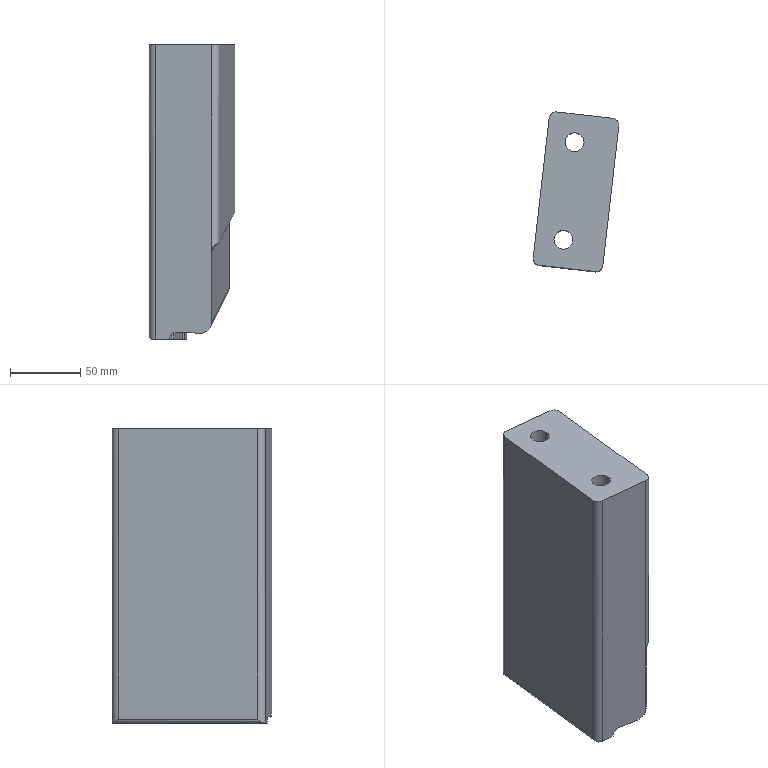Part | NX | features solid 2 | 1 solid | 30 faces | box 61.066 x 113.889 x 210 mm | volume 956028 mm3 | cylinder 15 | plane 14 | cone 1 | commonest cylinder face diameters 10 x7 13.5 x2 20 x2 6 x1 8.5 x1 9 x1
STEP:
#1=CARTESIAN_POINT('',(2372.499,-272.308,-109.613));
#2=VERTEX_POINT('',#1);
#3=CARTESIAN_POINT('',(2366.536,-324.649,-121.614));
#4=VERTEX_POINT('',#3);
#5=CARTESIAN_POINT('',(2363.422,-351.978,-127.881));
#6=DIRECTION('',(-0.1104,-0.9687,-0.2221));
#7=VECTOR('',#6,1000.);
#8=LINE('',#5,#7);
#9=EDGE_CURVE('',#2,#4,#8,.T.);
#10=ORIENTED_EDGE('',*,*,#9,.F.);
#11=CARTESIAN_POINT('',(2377.51,-274.226,-104.793));
#12=VERTEX_POINT('',#11);
#13=CARTESIAN_POINT('',(2372.499,-272.308,-109.613));
#14=CARTESIAN_POINT('',(2372.499,-272.308,-108.251));
#15=CARTESIAN_POINT('',(2373.556,-273.191,-105.664));
#16=CARTESIAN_POINT('',(2376.156,-274.098,-104.745));
#17=CARTESIAN_POINT('',(2377.51,-274.226,-104.793));
#18=B_SPLINE_CURVE_WITH_KNOTS('',3,(#13,#14,#15,#16,#17),.UNSPECIFIED.,.F.,.F.,(4,1,4),(0.,0.004026,0.008053),.UNSPECIFIED.);
#19=EDGE_CURVE('',#2,#12,#18,.T.);
#20=ORIENTED_EDGE('',*,*,#19,.T.);
#21=CARTESIAN_POINT('',(2371.85,-323.908,-116.185));
#22=VERTEX_POINT('',#21);
#23=CARTESIAN_POINT('',(2380.911,-244.376,-97.949));
#24=DIRECTION('',(0.1104,0.9687,0.2221));
#25=VECTOR('',#24,1000.);
#26=LINE('',#23,#25);
#27=EDGE_CURVE('',#22,#12,#26,.T.);
#28=ORIENTED_EDGE('',*,*,#27,.F.);
#29=CARTESIAN_POINT('',(2371.85,-323.908,-116.185));
#30=CARTESIAN_POINT('',(2370.434,-323.719,-116.122));
#31=CARTESIAN_POINT('',(2367.696,-324.057,-117.462));
#32=CARTESIAN_POINT('',(2366.536,-324.649,-120.186));
#33=CARTESIAN_POINT('',(2366.536,-324.649,-121.614));
#34=B_SPLINE_CURVE_WITH_KNOTS('',3,(#29,#30,#31,#32,#33),.UNSPECIFIED.,.F.,.F.,(4,1,4),(0.,0.004221,0.008443),.UNSPECIFIED.);
#35=EDGE_CURVE('',#22,#4,#34,.T.);
#36=ORIENTED_EDGE('',*,*,#35,.T.);
#37=EDGE_LOOP('',(#10,#20,#28,#36));
#38=FACE_BOUND('',#37,.T.);
#39=CARTESIAN_POINT('',(2377.356,-273.855,-109.838));
#40=DIRECTION('',(0.1104,0.9687,0.2221));
#41=DIRECTION('',(0.,0.2235,-0.9747));
#42=AXIS2_PLACEMENT_3D('',#39,#40,#41);
#43=CYLINDRICAL_SURFACE('',#42,5.);
#44=ADVANCED_FACE('',(#38),#43,.F.);
#45=CARTESIAN_POINT('',(2366.536,-324.649,-128.));
#46=VERTEX_POINT('',#45);
#47=CARTESIAN_POINT('',(2372.499,-272.308,-128.));
#48=VERTEX_POINT('',#47);
#49=CARTESIAN_POINT('',(2369.518,-298.479,-128.));
#50=DIRECTION('',(0.1132,0.9936,0.));
#51=VECTOR('',#50,1000.);
#52=LINE('',#49,#51);
#53=EDGE_CURVE('',#46,#48,#52,.T.);
#54=ORIENTED_EDGE('',*,*,#53,.T.);
#55=CARTESIAN_POINT('',(2372.499,-272.308,-101.));
#56=DIRECTION('',(0.,0.,1.));
#57=VECTOR('',#56,1000.);
#58=LINE('',#55,#57);
#59=EDGE_CURVE('',#48,#2,#58,.T.);
#60=ORIENTED_EDGE('',*,*,#59,.T.);
#61=ORIENTED_EDGE('',*,*,#9,.T.);
#62=CARTESIAN_POINT('',(2366.536,-324.649,-101.));
#63=DIRECTION('',(0.,0.,-1.));
#64=VECTOR('',#63,1000.);
#65=LINE('',#62,#64);
#66=EDGE_CURVE('',#4,#46,#65,.T.);
#67=ORIENTED_EDGE('',*,*,#66,.T.);
#68=EDGE_LOOP('',(#54,#60,#61,#67));
#69=FACE_BOUND('',#68,.T.);
#70=CARTESIAN_POINT('',(2369.518,-298.479,1.445));
#71=DIRECTION('',(-0.9936,0.1132,0.));
#72=DIRECTION('',(0.1132,0.9936,0.));
#73=AXIS2_PLACEMENT_3D('',#70,#71,#72);
#74=PLANE('',#73);
#75=ADVANCED_FACE('',(#69),#74,.F.);
#76=CARTESIAN_POINT('',(2363.363,-352.498,-128.));
#77=VERTEX_POINT('',#76);
#78=CARTESIAN_POINT('',(2364.575,-341.858,-128.));
#79=VERTEX_POINT('',#78);
#80=CARTESIAN_POINT('',(2369.518,-298.479,-128.));
#81=DIRECTION('',(0.1132,0.9936,0.));
#82=VECTOR('',#81,1000.);
#83=LINE('',#80,#82);
#84=EDGE_CURVE('',#77,#79,#83,.T.);
#85=ORIENTED_EDGE('',*,*,#84,.T.);
#86=CARTESIAN_POINT('',(2364.575,-341.858,-125.56));
#87=VERTEX_POINT('',#86);
#88=CARTESIAN_POINT('',(2364.575,-341.858,-101.));
#89=DIRECTION('',(0.,0.,1.));
#90=VECTOR('',#89,1000.);
#91=LINE('',#88,#90);
#92=EDGE_CURVE('',#79,#87,#91,.T.);
#93=ORIENTED_EDGE('',*,*,#92,.T.);
#94=CARTESIAN_POINT('',(2363.422,-351.978,-127.881));
#95=DIRECTION('',(-0.1104,-0.9687,-0.2221));
#96=VECTOR('',#95,1000.);
#97=LINE('',#94,#96);
#98=EDGE_CURVE('',#87,#77,#97,.T.);
#99=ORIENTED_EDGE('',*,*,#98,.T.);
#100=EDGE_LOOP('',(#85,#93,#99));
#101=FACE_BOUND('',#100,.T.);
#102=CARTESIAN_POINT('',(2369.518,-298.479,1.445));
#103=DIRECTION('',(-0.9936,0.1132,0.));
#104=DIRECTION('',(0.1132,0.9936,0.));
#105=AXIS2_PLACEMENT_3D('',#102,#103,#104);
#106=PLANE('',#105);
#107=ADVANCED_FACE('',(#101),#106,.F.);
#108=CARTESIAN_POINT('',(2379.774,-254.358,-100.238));
#109=VERTEX_POINT('',#108);
#110=CARTESIAN_POINT('',(2380.906,-244.421,-97.959));
#111=VERTEX_POINT('',#110);
#112=CARTESIAN_POINT('',(2380.911,-244.376,-97.949));
#113=DIRECTION('',(0.1104,0.9687,0.2221));
#114=VECTOR('',#113,1000.);
#115=LINE('',#112,#114);
#116=EDGE_CURVE('',#109,#111,#115,.T.);
#117=ORIENTED_EDGE('',*,*,#116,.F.);
#118=CARTESIAN_POINT('',(2374.46,-255.099,-105.667));
#119=VERTEX_POINT('',#118);
#120=CARTESIAN_POINT('',(2379.774,-254.358,-100.238));
#121=CARTESIAN_POINT('',(2378.358,-254.169,-100.174));
#122=CARTESIAN_POINT('',(2375.62,-254.507,-101.515));
#123=CARTESIAN_POINT('',(2374.46,-255.099,-104.238));
#124=CARTESIAN_POINT('',(2374.46,-255.099,-105.667));
#125=B_SPLINE_CURVE_WITH_KNOTS('',3,(#120,#121,#122,#123,#124),.UNSPECIFIED.,.F.,.F.,(4,1,4),(0.,0.004221,0.008443),.UNSPECIFIED.);
#126=EDGE_CURVE('',#109,#119,#125,.T.);
#127=ORIENTED_EDGE('',*,*,#126,.T.);
#128=CARTESIAN_POINT('',(2375.744,-243.832,-103.083));
#129=VERTEX_POINT('',#128);
#130=CARTESIAN_POINT('',(2363.422,-351.978,-127.881));
#131=DIRECTION('',(-0.1104,-0.9687,-0.2221));
#132=VECTOR('',#131,1000.);
#133=LINE('',#130,#132);
#134=EDGE_CURVE('',#129,#119,#133,.T.);
#135=ORIENTED_EDGE('',*,*,#134,.F.);
#136=CARTESIAN_POINT('',(2380.712,-244.398,-103.083));
#137=DIRECTION('',(-0.1132,-0.9936,0.));
#138=DIRECTION('',(0.,0.,1.));
#139=AXIS2_PLACEMENT_3D('',#136,#137,#138);
#140=ELLIPSE('',#139,5.128,5.);
#141=EDGE_CURVE('',#111,#129,#140,.T.);
#142=ORIENTED_EDGE('',*,*,#141,.F.);
#143=EDGE_LOOP('',(#117,#127,#135,#142));
#144=FACE_BOUND('',#143,.T.);
#145=CARTESIAN_POINT('',(2377.356,-273.855,-109.838));
#146=DIRECTION('',(0.1104,0.9687,0.2221));
#147=DIRECTION('',(0.,0.2235,-0.9747));
#148=AXIS2_PLACEMENT_3D('',#145,#146,#147);
#149=CYLINDRICAL_SURFACE('',#148,5.);
#150=ADVANCED_FACE('',(#144),#149,.F.);
#151=CARTESIAN_POINT('',(2393.099,-356.521,-118.358));
#152=VERTEX_POINT('',#151);
#153=CARTESIAN_POINT('',(2393.099,-356.521,82.));
#154=VERTEX_POINT('',#153);
#155=CARTESIAN_POINT('',(2393.099,-356.521,38.4));
#156=DIRECTION('',(0.,0.,1.));
#157=VECTOR('',#156,1000.);
#158=LINE('',#155,#157);
#159=EDGE_CURVE('',#152,#154,#158,.T.);
#160=ORIENTED_EDGE('',*,*,#159,.T.);
#161=CARTESIAN_POINT('',(2353.356,-351.993,82.));
#162=VERTEX_POINT('',#161);
#163=CARTESIAN_POINT('',(2417.456,-359.297,82.));
#164=DIRECTION('',(-0.9936,0.1132,0.));
#165=VECTOR('',#164,1000.);
#166=LINE('',#163,#165);
#167=EDGE_CURVE('',#154,#162,#166,.T.);
#168=ORIENTED_EDGE('',*,*,#167,.T.);
#169=CARTESIAN_POINT('',(2353.356,-351.993,-128.));
#170=VERTEX_POINT('',#169);
#171=CARTESIAN_POINT('',(2353.356,-351.993,-122.61));
#172=DIRECTION('',(0.,0.,-1.));
#173=VECTOR('',#172,1000.);
#174=LINE('',#171,#173);
#175=EDGE_CURVE('',#162,#170,#174,.T.);
#176=ORIENTED_EDGE('',*,*,#175,.T.);
#177=CARTESIAN_POINT('',(2363.293,-353.125,-128.));
#178=VERTEX_POINT('',#177);
#179=CARTESIAN_POINT('',(2417.456,-359.297,-128.));
#180=DIRECTION('',(-0.9936,0.1132,0.));
#181=VECTOR('',#180,1000.);
#182=LINE('',#179,#181);
#183=EDGE_CURVE('',#178,#170,#182,.T.);
#184=ORIENTED_EDGE('',*,*,#183,.F.);
#185=CARTESIAN_POINT('',(2368.454,-353.713,-123.02));
#186=VERTEX_POINT('',#185);
#187=CARTESIAN_POINT('',(2368.259,-353.691,-128.144));
#188=DIRECTION('',(0.1132,0.9936,0.));
#189=DIRECTION('',(0.,0.,1.));
#190=AXIS2_PLACEMENT_3D('',#187,#188,#189);
#191=ELLIPSE('',#190,5.128,5.);
#192=EDGE_CURVE('',#178,#186,#191,.T.);
#193=ORIENTED_EDGE('',*,*,#192,.T.);
#194=CARTESIAN_POINT('',(2385.336,-355.637,-123.702));
#195=VERTEX_POINT('',#194);
#196=CARTESIAN_POINT('',(2410.945,-358.555,-124.738));
#197=DIRECTION('',(-0.9928,0.1131,0.04014));
#198=VECTOR('',#197,1000.);
#199=LINE('',#196,#198);
#200=EDGE_CURVE('',#195,#186,#199,.T.);
#201=ORIENTED_EDGE('',*,*,#200,.F.);
#202=CARTESIAN_POINT('',(2385.647,-355.672,-115.504));
#203=DIRECTION('',(-0.1132,-0.9936,0.));
#204=DIRECTION('',(0.,0.,-1.));
#205=AXIS2_PLACEMENT_3D('',#202,#203,#204);
#206=ELLIPSE('',#205,8.205,8.);
#207=EDGE_CURVE('',#195,#152,#206,.T.);
#208=ORIENTED_EDGE('',*,*,#207,.T.);
#209=EDGE_LOOP('',(#160,#168,#176,#184,#193,#201,#208));
#210=FACE_BOUND('',#209,.T.);
#211=CARTESIAN_POINT('',(2417.456,-359.297,38.4));
#212=DIRECTION('',(0.1132,0.9936,0.));
#213=DIRECTION('',(0.,0.,1.));
#214=AXIS2_PLACEMENT_3D('',#211,#212,#213);
#215=PLANE('',#214);
#216=ADVANCED_FACE('',(#210),#215,.F.);
#217=CARTESIAN_POINT('',(2405.551,-247.228,82.));
#218=VERTEX_POINT('',#217);
#219=CARTESIAN_POINT('',(2365.808,-242.7,82.));
#220=VERTEX_POINT('',#219);
#221=CARTESIAN_POINT('',(2429.909,-250.004,82.));
#222=DIRECTION('',(-0.9936,0.1132,0.));
#223=VECTOR('',#222,1000.);
#224=LINE('',#221,#223);
#225=EDGE_CURVE('',#218,#220,#224,.T.);
#226=ORIENTED_EDGE('',*,*,#225,.F.);
#227=CARTESIAN_POINT('',(2405.551,-247.228,-93.298));
#228=VERTEX_POINT('',#227);
#229=CARTESIAN_POINT('',(2405.551,-247.228,-35.47));
#230=DIRECTION('',(0.,0.,-1.));
#231=VECTOR('',#230,1000.);
#232=LINE('',#229,#231);
#233=EDGE_CURVE('',#218,#228,#232,.T.);
#234=ORIENTED_EDGE('',*,*,#233,.T.);
#235=CARTESIAN_POINT('',(2397.788,-246.344,-98.642));
#236=VERTEX_POINT('',#235);
#237=CARTESIAN_POINT('',(2398.099,-246.379,-90.443));
#238=DIRECTION('',(-0.1132,-0.9936,0.));
#239=DIRECTION('',(0.,0.,-1.));
#240=AXIS2_PLACEMENT_3D('',#237,#238,#239);
#241=ELLIPSE('',#240,8.205,8.);
#242=EDGE_CURVE('',#236,#228,#241,.T.);
#243=ORIENTED_EDGE('',*,*,#242,.F.);
#244=CARTESIAN_POINT('',(2424.396,-249.376,-99.718));
#245=DIRECTION('',(-0.9928,0.1131,0.04014));
#246=VECTOR('',#245,1000.);
#247=LINE('',#244,#246);
#248=EDGE_CURVE('',#236,#111,#247,.T.);
#249=ORIENTED_EDGE('',*,*,#248,.T.);
#250=ORIENTED_EDGE('',*,*,#141,.T.);
#251=CARTESIAN_POINT('',(2375.744,-243.832,-128.));
#252=VERTEX_POINT('',#251);
#253=CARTESIAN_POINT('',(2375.744,-243.832,38.4));
#254=DIRECTION('',(0.,0.,1.));
#255=VECTOR('',#254,1000.);
#256=LINE('',#253,#255);
#257=EDGE_CURVE('',#252,#129,#256,.T.);
#258=ORIENTED_EDGE('',*,*,#257,.F.);
#259=CARTESIAN_POINT('',(2365.808,-242.7,-128.));
#260=VERTEX_POINT('',#259);
#261=CARTESIAN_POINT('',(2429.909,-250.004,-128.));
#262=DIRECTION('',(-0.9936,0.1132,0.));
#263=VECTOR('',#262,1000.);
#264=LINE('',#261,#263);
#265=EDGE_CURVE('',#252,#260,#264,.T.);
#266=ORIENTED_EDGE('',*,*,#265,.T.);
#267=CARTESIAN_POINT('',(2365.808,-242.7,38.4));
#268=DIRECTION('',(0.,0.,1.));
#269=VECTOR('',#268,1000.);
#270=LINE('',#267,#269);
#271=EDGE_CURVE('',#260,#220,#270,.T.);
#272=ORIENTED_EDGE('',*,*,#271,.T.);
#273=EDGE_LOOP('',(#226,#234,#243,#249,#250,#258,#266,#272));
#274=FACE_BOUND('',#273,.T.);
#275=CARTESIAN_POINT('',(2429.909,-250.004,38.4));
#276=DIRECTION('',(0.1132,0.9936,0.));
#277=DIRECTION('',(0.,0.,1.));
#278=AXIS2_PLACEMENT_3D('',#275,#276,#277);
#279=PLANE('',#278);
#280=ADVANCED_FACE('',(#274),#279,.T.);
#281=CARTESIAN_POINT('',(2409.953,-252.762,-36.609));
#282=VERTEX_POINT('',#281);
#283=CARTESIAN_POINT('',(2409.953,-252.762,82.));
#284=VERTEX_POINT('',#283);
#285=CARTESIAN_POINT('',(2409.953,-252.762,35.));
#286=DIRECTION('',(0.,0.,1.));
#287=VECTOR('',#286,1000.);
#288=LINE('',#285,#287);
#289=EDGE_CURVE('',#282,#284,#288,.T.);
#290=ORIENTED_EDGE('',*,*,#289,.T.);
#291=CARTESIAN_POINT('',(2398.633,-352.119,82.));
#292=VERTEX_POINT('',#291);
#293=CARTESIAN_POINT('',(2399.199,-347.152,82.));
#294=DIRECTION('',(-0.1132,-0.9936,0.));
#295=VECTOR('',#294,1000.);
#296=LINE('',#293,#295);
#297=EDGE_CURVE('',#284,#292,#296,.T.);
#298=ORIENTED_EDGE('',*,*,#297,.T.);
#299=CARTESIAN_POINT('',(2398.633,-352.119,-59.391));
#300=VERTEX_POINT('',#299);
#301=CARTESIAN_POINT('',(2398.633,-352.119,38.4));
#302=DIRECTION('',(0.,0.,-1.));
#303=VECTOR('',#302,1000.);
#304=LINE('',#301,#303);
#305=EDGE_CURVE('',#292,#300,#304,.T.);
#306=ORIENTED_EDGE('',*,*,#305,.T.);
#307=CARTESIAN_POINT('',(2401.568,-326.353,-53.483));
#308=DIRECTION('',(0.1104,0.9687,0.2221));
#309=VECTOR('',#308,1000.);
#310=LINE('',#307,#309);
#311=EDGE_CURVE('',#300,#282,#310,.T.);
#312=ORIENTED_EDGE('',*,*,#311,.T.);
#313=EDGE_LOOP('',(#290,#298,#306,#312));
#314=FACE_BOUND('',#313,.T.);
#315=CARTESIAN_POINT('',(2399.199,-347.152,38.4));
#316=DIRECTION('',(0.9936,-0.1132,0.));
#317=DIRECTION('',(-0.1132,-0.9936,0.));
#318=AXIS2_PLACEMENT_3D('',#315,#316,#317);
#319=PLANE('',#318);
#320=ADVANCED_FACE('',(#314),#319,.T.);
#321=ORIENTED_EDGE('',*,*,#233,.F.);
#322=CARTESIAN_POINT('',(2404.985,-252.196,82.));
#323=DIRECTION('',(0.,0.,-1.));
#324=DIRECTION('',(1.,0.,0.));
#325=AXIS2_PLACEMENT_3D('',#322,#323,#324);
#326=CIRCLE('',#325,5.);
#327=EDGE_CURVE('',#218,#284,#326,.T.);
#328=ORIENTED_EDGE('',*,*,#327,.T.);
#329=ORIENTED_EDGE('',*,*,#289,.F.);
#330=CARTESIAN_POINT('',(2409.957,-252.723,-36.6));
#331=VERTEX_POINT('',#330);
#332=CARTESIAN_POINT('',(2404.985,-252.196,-36.609));
#333=DIRECTION('',(0.02515,0.2207,-0.975));
#334=DIRECTION('',(-0.1104,-0.9687,-0.2221));
#335=AXIS2_PLACEMENT_3D('',#332,#333,#334);
#336=ELLIPSE('',#335,5.128,5.);
#337=EDGE_CURVE('',#331,#282,#336,.T.);
#338=ORIENTED_EDGE('',*,*,#337,.F.);
#339=CARTESIAN_POINT('',(2406.045,-247.31,-40.091));
#340=VERTEX_POINT('',#339);
#341=CARTESIAN_POINT('',(2406.045,-247.31,-40.091));
#342=CARTESIAN_POINT('',(2406.045,-247.31,-39.27));
#343=CARTESIAN_POINT('',(2406.446,-247.354,-37.641));
#344=CARTESIAN_POINT('',(2408.3,-248.195,-35.955));
#345=CARTESIAN_POINT('',(2409.846,-250.315,-36.028));
#346=CARTESIAN_POINT('',(2410.041,-251.926,-36.418));
#347=CARTESIAN_POINT('',(2409.957,-252.723,-36.6));
#348=B_SPLINE_CURVE_WITH_KNOTS('',3,(#341,#342,#343,#344,#345,#346,#347),.UNSPECIFIED.,.F.,.F.,(4,1,1,1,4),(0.,0.00243,0.004861,0.007291,0.009722),.UNSPECIFIED.);
#349=EDGE_CURVE('',#340,#331,#348,.T.);
#350=ORIENTED_EDGE('',*,*,#349,.F.);
#351=CARTESIAN_POINT('',(2406.045,-247.31,-90.449));
#352=VERTEX_POINT('',#351);
#353=CARTESIAN_POINT('',(2406.045,-247.31,-90.449));
#354=CARTESIAN_POINT('',(2406.045,-247.31,-87.116));
#355=CARTESIAN_POINT('',(2406.045,-247.31,-83.782));
#356=CARTESIAN_POINT('',(2406.045,-247.31,-66.996));
#357=CARTESIAN_POINT('',(2406.045,-247.31,-53.544));
#358=CARTESIAN_POINT('',(2406.045,-247.31,-40.091));
#359=B_SPLINE_CURVE_WITH_KNOTS('',3,(#353,#354,#355,#356,#357,#358),.UNSPECIFIED.,.F.,.F.,(4,2,4),(0.,0.1986,1.),.UNSPECIFIED.);
#360=EDGE_CURVE('',#352,#340,#359,.T.);
#361=ORIENTED_EDGE('',*,*,#360,.F.);
#362=CARTESIAN_POINT('',(2405.551,-247.228,-93.298));
#363=CARTESIAN_POINT('',(2405.881,-247.266,-92.38));
#364=CARTESIAN_POINT('',(2406.045,-247.31,-91.425));
#365=CARTESIAN_POINT('',(2406.045,-247.31,-90.449));
#366=B_SPLINE_CURVE_WITH_KNOTS('',3,(#362,#363,#364,#365),.UNSPECIFIED.,.F.,.F.,(4,4),(0.,0.002893),.UNSPECIFIED.);
#367=EDGE_CURVE('',#228,#352,#366,.T.);
#368=ORIENTED_EDGE('',*,*,#367,.F.);
#369=EDGE_LOOP('',(#321,#328,#329,#338,#350,#361,#368));
#370=FACE_BOUND('',#369,.T.);
#371=CARTESIAN_POINT('',(2404.985,-252.196,38.4));
#372=DIRECTION('',(0.,0.,-1.));
#373=DIRECTION('',(0.,-1.,0.));
#374=AXIS2_PLACEMENT_3D('',#371,#372,#373);
#375=CYLINDRICAL_SURFACE('',#374,5.);
#376=ADVANCED_FACE('',(#370),#375,.T.);
#377=ORIENTED_EDGE('',*,*,#305,.F.);
#378=CARTESIAN_POINT('',(2393.665,-351.553,82.));
#379=DIRECTION('',(0.,0.,-1.));
#380=DIRECTION('',(1.,0.,0.));
#381=AXIS2_PLACEMENT_3D('',#378,#379,#380);
#382=CIRCLE('',#381,5.);
#383=EDGE_CURVE('',#292,#154,#382,.T.);
#384=ORIENTED_EDGE('',*,*,#383,.T.);
#385=ORIENTED_EDGE('',*,*,#159,.F.);
#386=CARTESIAN_POINT('',(2393.598,-356.553,-115.498));
#387=VERTEX_POINT('',#386);
#388=CARTESIAN_POINT('',(2393.598,-356.553,-115.498));
#389=CARTESIAN_POINT('',(2393.598,-356.553,-116.477));
#390=CARTESIAN_POINT('',(2393.43,-356.559,-117.437));
#391=CARTESIAN_POINT('',(2393.099,-356.521,-118.358));
#392=B_SPLINE_CURVE_WITH_KNOTS('',3,(#388,#389,#390,#391),.UNSPECIFIED.,.F.,.F.,(4,4),(0.,0.002905),.UNSPECIFIED.);
#393=EDGE_CURVE('',#387,#152,#392,.T.);
#394=ORIENTED_EDGE('',*,*,#393,.F.);
#395=CARTESIAN_POINT('',(2393.598,-356.553,-65.14));
#396=VERTEX_POINT('',#395);
#397=CARTESIAN_POINT('',(2393.598,-356.553,-65.14));
#398=CARTESIAN_POINT('',(2393.598,-356.553,-68.473));
#399=CARTESIAN_POINT('',(2393.598,-356.553,-71.807));
#400=CARTESIAN_POINT('',(2393.598,-356.553,-88.593));
#401=CARTESIAN_POINT('',(2393.598,-356.553,-102.045));
#402=CARTESIAN_POINT('',(2393.598,-356.553,-115.498));
#403=B_SPLINE_CURVE_WITH_KNOTS('',3,(#397,#398,#399,#400,#401,#402),.UNSPECIFIED.,.F.,.F.,(4,2,4),(0.,0.1986,1.),.UNSPECIFIED.);
#404=EDGE_CURVE('',#396,#387,#403,.T.);
#405=ORIENTED_EDGE('',*,*,#404,.F.);
#406=CARTESIAN_POINT('',(2398.628,-352.159,-59.4));
#407=VERTEX_POINT('',#406);
#408=CARTESIAN_POINT('',(2398.628,-352.159,-59.4));
#409=CARTESIAN_POINT('',(2398.526,-352.99,-59.591));
#410=CARTESIAN_POINT('',(2397.908,-354.581,-59.936));
#411=CARTESIAN_POINT('',(2395.971,-356.186,-60.757));
#412=CARTESIAN_POINT('',(2394.07,-356.596,-62.585));
#413=CARTESIAN_POINT('',(2393.598,-356.553,-64.28));
#414=CARTESIAN_POINT('',(2393.598,-356.553,-65.14));
#415=B_SPLINE_CURVE_WITH_KNOTS('',3,(#408,#409,#410,#411,#412,#413,#414),.UNSPECIFIED.,.F.,.F.,(4,1,1,1,4),(0.,0.002539,0.005079,0.007618,0.01016),.UNSPECIFIED.);
#416=EDGE_CURVE('',#407,#396,#415,.T.);
#417=ORIENTED_EDGE('',*,*,#416,.F.);
#418=CARTESIAN_POINT('',(2393.665,-351.553,-59.391));
#419=DIRECTION('',(0.02515,0.2207,-0.975));
#420=DIRECTION('',(0.1104,0.9687,0.2221));
#421=AXIS2_PLACEMENT_3D('',#418,#419,#420);
#422=ELLIPSE('',#421,5.128,5.);
#423=EDGE_CURVE('',#300,#407,#422,.T.);
#424=ORIENTED_EDGE('',*,*,#423,.F.);
#425=EDGE_LOOP('',(#377,#384,#385,#394,#405,#417,#424));
#426=FACE_BOUND('',#425,.T.);
#427=CARTESIAN_POINT('',(2393.665,-351.553,38.4));
#428=DIRECTION('',(0.,0.,1.));
#429=DIRECTION('',(0.,1.,0.));
#430=AXIS2_PLACEMENT_3D('',#427,#428,#429);
#431=CYLINDRICAL_SURFACE('',#430,5.);
#432=ADVANCED_FACE('',(#426),#431,.T.);
#433=CARTESIAN_POINT('',(2360.274,-247.102,82.));
#434=VERTEX_POINT('',#433);
#435=CARTESIAN_POINT('',(2348.954,-346.459,82.));
#436=VERTEX_POINT('',#435);
#437=CARTESIAN_POINT('',(2349.52,-341.491,82.));
#438=DIRECTION('',(-0.1132,-0.9936,0.));
#439=VECTOR('',#438,1000.);
#440=LINE('',#437,#439);
#441=EDGE_CURVE('',#434,#436,#440,.T.);
#442=ORIENTED_EDGE('',*,*,#441,.F.);
#443=CARTESIAN_POINT('',(2360.274,-247.102,-125.));
#444=VERTEX_POINT('',#443);
#445=CARTESIAN_POINT('',(2360.274,-247.102,38.4));
#446=DIRECTION('',(0.,0.,-1.));
#447=VECTOR('',#446,1000.);
#448=LINE('',#445,#447);
#449=EDGE_CURVE('',#434,#444,#448,.T.);
#450=ORIENTED_EDGE('',*,*,#449,.T.);
#451=CARTESIAN_POINT('',(2348.954,-346.459,-125.));
#452=VERTEX_POINT('',#451);
#453=CARTESIAN_POINT('',(2349.52,-341.491,-125.));
#454=DIRECTION('',(-0.1132,-0.9936,0.));
#455=VECTOR('',#454,1000.);
#456=LINE('',#453,#455);
#457=EDGE_CURVE('',#444,#452,#456,.T.);
#458=ORIENTED_EDGE('',*,*,#457,.T.);
#459=CARTESIAN_POINT('',(2348.954,-346.459,35.));
#460=DIRECTION('',(0.,0.,1.));
#461=VECTOR('',#460,1000.);
#462=LINE('',#459,#461);
#463=EDGE_CURVE('',#452,#436,#462,.T.);
#464=ORIENTED_EDGE('',*,*,#463,.T.);
#465=EDGE_LOOP('',(#442,#450,#458,#464));
#466=FACE_BOUND('',#465,.T.);
#467=CARTESIAN_POINT('',(2349.52,-341.491,38.4));
#468=DIRECTION('',(0.9936,-0.1132,0.));
#469=DIRECTION('',(-0.1132,-0.9936,0.));
#470=AXIS2_PLACEMENT_3D('',#467,#468,#469);
#471=PLANE('',#470);
#472=ADVANCED_FACE('',(#466),#471,.F.);
#473=ORIENTED_EDGE('',*,*,#449,.F.);
#474=CARTESIAN_POINT('',(2365.242,-247.668,82.));
#475=DIRECTION('',(0.,0.,-1.));
#476=DIRECTION('',(1.,0.,0.));
#477=AXIS2_PLACEMENT_3D('',#474,#475,#476);
#478=CIRCLE('',#477,5.);
#479=EDGE_CURVE('',#434,#220,#478,.T.);
#480=ORIENTED_EDGE('',*,*,#479,.T.);
#481=ORIENTED_EDGE('',*,*,#271,.F.);
#482=CARTESIAN_POINT('',(2363.774,-242.889,-128.));
#483=VERTEX_POINT('',#482);
#484=CARTESIAN_POINT('',(2365.242,-247.668,-128.));
#485=DIRECTION('',(0.,0.,-1.));
#486=DIRECTION('',(-1.,0.,0.));
#487=AXIS2_PLACEMENT_3D('',#484,#485,#486);
#488=CIRCLE('',#487,5.);
#489=EDGE_CURVE('',#483,#260,#488,.T.);
#490=ORIENTED_EDGE('',*,*,#489,.F.);
#491=CARTESIAN_POINT('',(2363.774,-242.889,-128.));
#492=CARTESIAN_POINT('',(2362.701,-243.218,-128.));
#493=CARTESIAN_POINT('',(2360.996,-244.545,-127.03));
#494=CARTESIAN_POINT('',(2360.373,-246.235,-125.676));
#495=CARTESIAN_POINT('',(2360.274,-247.102,-125.));
#496=B_SPLINE_CURVE_WITH_KNOTS('',3,(#491,#492,#493,#494,#495),.UNSPECIFIED.,.F.,.F.,(4,1,4),(0.,0.00331,0.006621),.UNSPECIFIED.);
#497=EDGE_CURVE('',#483,#444,#496,.T.);
#498=ORIENTED_EDGE('',*,*,#497,.T.);
#499=EDGE_LOOP('',(#473,#480,#481,#490,#498));
#500=FACE_BOUND('',#499,.T.);
#501=CARTESIAN_POINT('',(2365.242,-247.668,38.4));
#502=DIRECTION('',(0.,0.,1.));
#503=DIRECTION('',(0.,1.,0.));
#504=AXIS2_PLACEMENT_3D('',#501,#502,#503);
#505=CYLINDRICAL_SURFACE('',#504,5.);
#506=ADVANCED_FACE('',(#500),#505,.T.);
#507=ORIENTED_EDGE('',*,*,#175,.F.);
#508=CARTESIAN_POINT('',(2353.922,-347.025,82.));
#509=DIRECTION('',(0.,0.,-1.));
#510=DIRECTION('',(1.,0.,0.));
#511=AXIS2_PLACEMENT_3D('',#508,#509,#510);
#512=CIRCLE('',#511,5.);
#513=EDGE_CURVE('',#162,#436,#512,.T.);
#514=ORIENTED_EDGE('',*,*,#513,.T.);
#515=ORIENTED_EDGE('',*,*,#463,.F.);
#516=CARTESIAN_POINT('',(2351.416,-351.352,-128.));
#517=VERTEX_POINT('',#516);
#518=CARTESIAN_POINT('',(2348.954,-346.459,-125.));
#519=CARTESIAN_POINT('',(2348.856,-347.321,-125.672));
#520=CARTESIAN_POINT('',(2349.076,-349.108,-127.028));
#521=CARTESIAN_POINT('',(2350.45,-350.793,-128.));
#522=CARTESIAN_POINT('',(2351.416,-351.352,-128.));
#523=B_SPLINE_CURVE_WITH_KNOTS('',3,(#518,#519,#520,#521,#522),.UNSPECIFIED.,.F.,.F.,(4,1,4),(-0.00001414,0.003277,0.006568),.UNSPECIFIED.);
#524=EDGE_CURVE('',#452,#517,#523,.T.);
#525=ORIENTED_EDGE('',*,*,#524,.T.);
#526=CARTESIAN_POINT('',(2353.922,-347.025,-128.));
#527=DIRECTION('',(0.,0.,-1.));
#528=DIRECTION('',(-1.,0.,0.));
#529=AXIS2_PLACEMENT_3D('',#526,#527,#528);
#530=CIRCLE('',#529,5.);
#531=EDGE_CURVE('',#170,#517,#530,.T.);
#532=ORIENTED_EDGE('',*,*,#531,.F.);
#533=EDGE_LOOP('',(#507,#514,#515,#525,#532));
#534=FACE_BOUND('',#533,.T.);
#535=CARTESIAN_POINT('',(2353.922,-347.025,38.4));
#536=DIRECTION('',(0.,0.,-1.));
#537=DIRECTION('',(0.,-1.,0.));
#538=AXIS2_PLACEMENT_3D('',#535,#536,#537);
#539=CYLINDRICAL_SURFACE('',#538,5.);
#540=ADVANCED_FACE('',(#534),#539,.T.);
#541=CARTESIAN_POINT('',(2380.805,-294.592,-109.543));
#542=VERTEX_POINT('',#541);
#543=CARTESIAN_POINT('',(2381.064,-298.834,-110.526));
#544=DIRECTION('',(0.01376,-0.225,0.9743));
#545=DIRECTION('',(-0.05948,0.9725,0.2254));
#546=AXIS2_PLACEMENT_3D('',#543,#544,#545);
#547=ELLIPSE('',#546,4.362,4.25);
#548=EDGE_CURVE('',#542,#542,#547,.T.);
#549=ORIENTED_EDGE('',*,*,#548,.T.);
#550=EDGE_LOOP('',(#549));
#551=FACE_BOUND('',#550,.T.);
#552=ORIENTED_EDGE('',*,*,#27,.T.);
#553=CARTESIAN_POINT('',(2378.448,-264.27,-102.508));
#554=DIRECTION('',(0.01376,-0.225,0.9743));
#555=DIRECTION('',(-0.05948,0.9725,0.2254));
#556=AXIS2_PLACEMENT_3D('',#553,#554,#555);
#557=ELLIPSE('',#556,10.264,10.);
#558=EDGE_CURVE('',#12,#109,#557,.T.);
#559=ORIENTED_EDGE('',*,*,#558,.T.);
#560=ORIENTED_EDGE('',*,*,#116,.T.);
#561=ORIENTED_EDGE('',*,*,#248,.F.);
#562=CARTESIAN_POINT('',(2399.334,-232.771,-95.53));
#563=DIRECTION('',(-0.1104,-0.9687,-0.2221));
#564=VECTOR('',#563,1000.);
#565=LINE('',#562,#564);
#566=EDGE_CURVE('',#236,#195,#565,.T.);
#567=ORIENTED_EDGE('',*,*,#566,.T.);
#568=ORIENTED_EDGE('',*,*,#200,.T.);
#569=CARTESIAN_POINT('',(2369.586,-343.776,-120.741));
#570=VERTEX_POINT('',#569);
#571=CARTESIAN_POINT('',(2380.911,-244.376,-97.949));
#572=DIRECTION('',(0.1104,0.9687,0.2221));
#573=VECTOR('',#572,1000.);
#574=LINE('',#571,#573);
#575=EDGE_CURVE('',#186,#570,#574,.T.);
#576=ORIENTED_EDGE('',*,*,#575,.T.);
#577=CARTESIAN_POINT('',(2370.523,-333.82,-118.455));
#578=DIRECTION('',(0.01376,-0.225,0.9743));
#579=DIRECTION('',(-0.05948,0.9725,0.2254));
#580=AXIS2_PLACEMENT_3D('',#577,#578,#579);
#581=ELLIPSE('',#580,10.264,10.);
#582=EDGE_CURVE('',#570,#22,#581,.T.);
#583=ORIENTED_EDGE('',*,*,#582,.T.);
#584=EDGE_LOOP('',(#552,#559,#560,#561,#567,#568,#576,#583));
#585=FACE_BOUND('',#584,.T.);
#586=CARTESIAN_POINT('',(2436.542,-222.854,-93.765));
#587=DIRECTION('',(0.01376,-0.225,0.9743));
#588=DIRECTION('',(-0.05948,0.9725,0.2254));
#589=AXIS2_PLACEMENT_3D('',#586,#587,#588);
#590=PLANE('',#589);
#591=ADVANCED_FACE('',(#551,#585),#590,.F.);
#592=CARTESIAN_POINT('',(2393.099,-360.929,-116.501));
#593=DIRECTION('',(0.1104,0.9687,0.2221));
#594=VECTOR('',#593,1000.);
#595=LINE('',#592,#594);
#596=EDGE_CURVE('',#387,#352,#595,.T.);
#597=ORIENTED_EDGE('',*,*,#596,.F.);
#598=ORIENTED_EDGE('',*,*,#393,.T.);
#599=ORIENTED_EDGE('',*,*,#207,.F.);
#600=ORIENTED_EDGE('',*,*,#566,.F.);
#601=ORIENTED_EDGE('',*,*,#242,.T.);
#602=ORIENTED_EDGE('',*,*,#367,.T.);
#603=EDGE_LOOP('',(#597,#598,#599,#600,#601,#602));
#604=FACE_BOUND('',#603,.T.);
#605=CARTESIAN_POINT('',(2401.001,-220.905,-84.602));
#606=DIRECTION('',(-0.1104,-0.9687,-0.2221));
#607=DIRECTION('',(0.,0.2235,-0.9747));
#608=AXIS2_PLACEMENT_3D('',#605,#606,#607);
#609=CYLINDRICAL_SURFACE('',#608,8.);
#610=ADVANCED_FACE('',(#604),#609,.T.);
#611=CARTESIAN_POINT('',(2407.715,-232.647,-36.729));
#612=DIRECTION('',(-0.1104,-0.9687,-0.2221));
#613=VECTOR('',#612,1000.);
#614=LINE('',#611,#613);
#615=EDGE_CURVE('',#340,#396,#614,.T.);
#616=ORIENTED_EDGE('',*,*,#615,.T.);
#617=ORIENTED_EDGE('',*,*,#404,.T.);
#618=ORIENTED_EDGE('',*,*,#596,.T.);
#619=ORIENTED_EDGE('',*,*,#360,.T.);
#620=EDGE_LOOP('',(#616,#617,#618,#619));
#621=FACE_BOUND('',#620,.T.);
#622=CARTESIAN_POINT('',(2407.602,-233.641,-32.341));
#623=DIRECTION('',(-0.9936,0.1132,0.000000002));
#624=DIRECTION('',(0.1132,0.9936,0.000000002));
#625=AXIS2_PLACEMENT_3D('',#622,#623,#624);
#626=PLANE('',#625);
#627=ADVANCED_FACE('',(#621),#626,.F.);
#628=CARTESIAN_POINT('',(2397.78,-359.603,-61.107));
#629=DIRECTION('',(0.1104,0.9687,0.2221));
#630=VECTOR('',#629,1000.);
#631=LINE('',#628,#630);
#632=EDGE_CURVE('',#407,#331,#631,.T.);
#633=ORIENTED_EDGE('',*,*,#632,.F.);
#634=ORIENTED_EDGE('',*,*,#416,.T.);
#635=ORIENTED_EDGE('',*,*,#615,.F.);
#636=ORIENTED_EDGE('',*,*,#349,.T.);
#637=EDGE_LOOP('',(#633,#634,#635,#636));
#638=FACE_BOUND('',#637,.T.);
#639=CARTESIAN_POINT('',(2397.059,-365.932,-67.174));
#640=DIRECTION('',(0.1104,0.9687,0.2221));
#641=DIRECTION('',(0.,-0.2235,0.9747));
#642=AXIS2_PLACEMENT_3D('',#639,#640,#641);
#643=CYLINDRICAL_SURFACE('',#642,4.5);
#644=ADVANCED_FACE('',(#638),#643,.F.);
#645=ORIENTED_EDGE('',*,*,#311,.F.);
#646=ORIENTED_EDGE('',*,*,#423,.T.);
#647=ORIENTED_EDGE('',*,*,#632,.T.);
#648=ORIENTED_EDGE('',*,*,#337,.T.);
#649=EDGE_LOOP('',(#645,#646,#647,#648));
#650=FACE_BOUND('',#649,.T.);
#651=CARTESIAN_POINT('',(2449.123,-372.87,-62.786));
#652=DIRECTION('',(0.02515,0.2207,-0.975));
#653=DIRECTION('',(-0.1104,-0.9687,-0.2221));
#654=AXIS2_PLACEMENT_3D('',#651,#652,#653);
#655=PLANE('',#654);
#656=ADVANCED_FACE('',(#650),#655,.T.);
#657=ORIENTED_EDGE('',*,*,#134,.T.);
#658=CARTESIAN_POINT('',(2374.46,-255.099,-128.));
#659=VERTEX_POINT('',#658);
#660=CARTESIAN_POINT('',(2374.46,-255.099,-101.));
#661=DIRECTION('',(0.,0.,-1.));
#662=VECTOR('',#661,1000.);
#663=LINE('',#660,#662);
#664=EDGE_CURVE('',#119,#659,#663,.T.);
#665=ORIENTED_EDGE('',*,*,#664,.T.);
#666=CARTESIAN_POINT('',(2369.518,-298.479,-128.));
#667=DIRECTION('',(0.1132,0.9936,0.));
#668=VECTOR('',#667,1000.);
#669=LINE('',#666,#668);
#670=EDGE_CURVE('',#659,#252,#669,.T.);
#671=ORIENTED_EDGE('',*,*,#670,.T.);
#672=ORIENTED_EDGE('',*,*,#257,.T.);
#673=EDGE_LOOP('',(#657,#665,#671,#672));
#674=FACE_BOUND('',#673,.T.);
#675=CARTESIAN_POINT('',(2369.518,-298.479,1.445));
#676=DIRECTION('',(-0.9936,0.1132,0.));
#677=DIRECTION('',(0.1132,0.9936,0.));
#678=AXIS2_PLACEMENT_3D('',#675,#676,#677);
#679=PLANE('',#678);
#680=ADVANCED_FACE('',(#674),#679,.F.);
#681=ORIENTED_EDGE('',*,*,#497,.F.);
#682=CARTESIAN_POINT('',(2369.029,-196.759,-128.));
#683=DIRECTION('',(0.1132,0.9936,0.));
#684=VECTOR('',#683,1000.);
#685=LINE('',#682,#684);
#686=EDGE_CURVE('',#517,#483,#685,.T.);
#687=ORIENTED_EDGE('',*,*,#686,.F.);
#688=ORIENTED_EDGE('',*,*,#524,.F.);
#689=ORIENTED_EDGE('',*,*,#457,.F.);
#690=EDGE_LOOP('',(#681,#687,#688,#689));
#691=FACE_BOUND('',#690,.T.);
#692=CARTESIAN_POINT('',(2369.029,-196.759,-125.));
#693=DIRECTION('',(-0.1132,-0.9936,0.));
#694=DIRECTION('',(-0.9936,0.1132,0.));
#695=AXIS2_PLACEMENT_3D('',#692,#693,#694);
#696=CYLINDRICAL_SURFACE('',#695,3.);
#697=ADVANCED_FACE('',(#691),#696,.T.);
#698=ORIENTED_EDGE('',*,*,#670,.F.);
#699=CARTESIAN_POINT('',(2378.448,-264.27,-128.));
#700=DIRECTION('',(0.,0.,1.));
#701=DIRECTION('',(-1.,0.,0.));
#702=AXIS2_PLACEMENT_3D('',#699,#700,#701);
#703=CIRCLE('',#702,10.);
#704=EDGE_CURVE('',#659,#48,#703,.T.);
#705=ORIENTED_EDGE('',*,*,#704,.T.);
#706=ORIENTED_EDGE('',*,*,#53,.F.);
#707=CARTESIAN_POINT('',(2370.523,-333.82,-128.));
#708=DIRECTION('',(0.,0.,1.));
#709=DIRECTION('',(-1.,0.,0.));
#710=AXIS2_PLACEMENT_3D('',#707,#708,#709);
#711=CIRCLE('',#710,10.);
#712=EDGE_CURVE('',#46,#79,#711,.T.);
#713=ORIENTED_EDGE('',*,*,#712,.T.);
#714=ORIENTED_EDGE('',*,*,#84,.F.);
#715=CARTESIAN_POINT('',(2368.331,-353.064,-128.));
#716=DIRECTION('',(0.,0.,1.));
#717=DIRECTION('',(0.1132,0.9936,0.));
#718=AXIS2_PLACEMENT_3D('',#715,#716,#717);
#719=ELLIPSE('',#718,22.509,5.);
#720=EDGE_CURVE('',#77,#178,#719,.T.);
#721=ORIENTED_EDGE('',*,*,#720,.T.);
#722=ORIENTED_EDGE('',*,*,#183,.T.);
#723=ORIENTED_EDGE('',*,*,#531,.T.);
#724=ORIENTED_EDGE('',*,*,#686,.T.);
#725=ORIENTED_EDGE('',*,*,#489,.T.);
#726=ORIENTED_EDGE('',*,*,#265,.F.);
#727=EDGE_LOOP('',(#698,#705,#706,#713,#714,#721,#722,#723,#724,#725,#726));
#728=FACE_BOUND('',#727,.T.);
#729=CARTESIAN_POINT('',(2535.468,-215.723,-128.));
#730=DIRECTION('',(0.,0.,-1.));
#731=DIRECTION('',(-0.1132,-0.9936,0.));
#732=AXIS2_PLACEMENT_3D('',#729,#730,#731);
#733=PLANE('',#732);
#734=ADVANCED_FACE('',(#728),#733,.T.);
#735=ORIENTED_EDGE('',*,*,#98,.F.);
#736=CARTESIAN_POINT('',(2364.575,-341.858,-125.56));
#737=CARTESIAN_POINT('',(2364.575,-341.858,-124.199));
#738=CARTESIAN_POINT('',(2365.632,-342.741,-121.611));
#739=CARTESIAN_POINT('',(2368.232,-343.648,-120.692));
#740=CARTESIAN_POINT('',(2369.586,-343.776,-120.741));
#741=B_SPLINE_CURVE_WITH_KNOTS('',3,(#736,#737,#738,#739,#740),.UNSPECIFIED.,.F.,.F.,(4,1,4),(0.,0.004026,0.008053),.UNSPECIFIED.);
#742=EDGE_CURVE('',#87,#570,#741,.T.);
#743=ORIENTED_EDGE('',*,*,#742,.T.);
#744=ORIENTED_EDGE('',*,*,#575,.F.);
#745=ORIENTED_EDGE('',*,*,#192,.F.);
#746=ORIENTED_EDGE('',*,*,#720,.F.);
#747=EDGE_LOOP('',(#735,#743,#744,#745,#746));
#748=FACE_BOUND('',#747,.T.);
#749=CARTESIAN_POINT('',(2377.356,-273.855,-109.838));
#750=DIRECTION('',(0.1104,0.9687,0.2221));
#751=DIRECTION('',(0.,0.2235,-0.9747));
#752=AXIS2_PLACEMENT_3D('',#749,#750,#751);
#753=CYLINDRICAL_SURFACE('',#752,5.);
#754=ADVANCED_FACE('',(#748),#753,.F.);
#755=CARTESIAN_POINT('',(2385.198,-264.27,82.));
#756=VERTEX_POINT('',#755);
#757=CARTESIAN_POINT('',(2378.448,-264.27,82.));
#758=DIRECTION('',(0.,0.,1.));
#759=DIRECTION('',(1.,0.,0.));
#760=AXIS2_PLACEMENT_3D('',#757,#758,#759);
#761=CIRCLE('',#760,6.75);
#762=EDGE_CURVE('',#756,#756,#761,.T.);
#763=ORIENTED_EDGE('',*,*,#762,.F.);
#764=EDGE_LOOP('',(#763));
#765=FACE_BOUND('',#764,.T.);
#766=CARTESIAN_POINT('',(2377.273,-333.82,82.));
#767=VERTEX_POINT('',#766);
#768=CARTESIAN_POINT('',(2370.523,-333.82,82.));
#769=DIRECTION('',(0.,0.,1.));
#770=DIRECTION('',(1.,0.,0.));
#771=AXIS2_PLACEMENT_3D('',#768,#769,#770);
#772=CIRCLE('',#771,6.75);
#773=EDGE_CURVE('',#767,#767,#772,.T.);
#774=ORIENTED_EDGE('',*,*,#773,.F.);
#775=EDGE_LOOP('',(#774));
#776=FACE_BOUND('',#775,.T.);
#777=ORIENTED_EDGE('',*,*,#327,.F.);
#778=ORIENTED_EDGE('',*,*,#225,.T.);
#779=ORIENTED_EDGE('',*,*,#479,.F.);
#780=ORIENTED_EDGE('',*,*,#441,.T.);
#781=ORIENTED_EDGE('',*,*,#513,.F.);
#782=ORIENTED_EDGE('',*,*,#167,.F.);
#783=ORIENTED_EDGE('',*,*,#383,.F.);
#784=ORIENTED_EDGE('',*,*,#297,.F.);
#785=EDGE_LOOP('',(#777,#778,#779,#780,#781,#782,#783,#784));
#786=FACE_BOUND('',#785,.T.);
#787=CARTESIAN_POINT('',(2439.558,-260.55,82.));
#788=DIRECTION('',(0.,0.,1.));
#789=DIRECTION('',(-1.,0.,0.));
#790=AXIS2_PLACEMENT_3D('',#787,#788,#789);
#791=PLANE('',#790);
#792=ADVANCED_FACE('',(#765,#776,#786),#791,.T.);
#793=CARTESIAN_POINT('',(2380.523,-333.82,2.));
#794=VERTEX_POINT('',#793);
#795=CARTESIAN_POINT('',(2370.523,-333.82,2.));
#796=DIRECTION('',(0.,0.,-1.));
#797=DIRECTION('',(1.,0.,0.));
#798=AXIS2_PLACEMENT_3D('',#795,#796,#797);
#799=CIRCLE('',#798,10.);
#800=EDGE_CURVE('',#794,#794,#799,.T.);
#801=ORIENTED_EDGE('',*,*,#800,.F.);
#802=EDGE_LOOP('',(#801));
#803=FACE_BOUND('',#802,.T.);
#804=ORIENTED_EDGE('',*,*,#35,.F.);
#805=ORIENTED_EDGE('',*,*,#582,.F.);
#806=ORIENTED_EDGE('',*,*,#742,.F.);
#807=ORIENTED_EDGE('',*,*,#92,.F.);
#808=ORIENTED_EDGE('',*,*,#712,.F.);
#809=ORIENTED_EDGE('',*,*,#66,.F.);
#810=EDGE_LOOP('',(#804,#805,#806,#807,#808,#809));
#811=FACE_BOUND('',#810,.T.);
#812=CARTESIAN_POINT('',(2370.523,-333.82,-101.));
#813=DIRECTION('',(0.,0.,1.));
#814=DIRECTION('',(-0.9744,0.225,0.));
#815=AXIS2_PLACEMENT_3D('',#812,#813,#814);
#816=CYLINDRICAL_SURFACE('',#815,10.);
#817=ADVANCED_FACE('',(#803,#811),#816,.F.);
#818=ORIENTED_EDGE('',*,*,#773,.T.);
#819=EDGE_LOOP('',(#818));
#820=FACE_BOUND('',#819,.T.);
#821=CARTESIAN_POINT('',(2377.273,-333.82,2.));
#822=VERTEX_POINT('',#821);
#823=CARTESIAN_POINT('',(2370.523,-333.82,2.));
#824=DIRECTION('',(0.,0.,-1.));
#825=DIRECTION('',(1.,0.,0.));
#826=AXIS2_PLACEMENT_3D('',#823,#824,#825);
#827=CIRCLE('',#826,6.75);
#828=EDGE_CURVE('',#822,#822,#827,.T.);
#829=ORIENTED_EDGE('',*,*,#828,.T.);
#830=EDGE_LOOP('',(#829));
#831=FACE_BOUND('',#830,.T.);
#832=CARTESIAN_POINT('',(2370.523,-333.82,-101.));
#833=DIRECTION('',(0.,0.,1.));
#834=DIRECTION('',(-0.9744,0.225,0.));
#835=AXIS2_PLACEMENT_3D('',#832,#833,#834);
#836=CYLINDRICAL_SURFACE('',#835,6.75);
#837=ADVANCED_FACE('',(#820,#831),#836,.F.);
#838=ORIENTED_EDGE('',*,*,#828,.F.);
#839=EDGE_LOOP('',(#838));
#840=FACE_BOUND('',#839,.T.);
#841=ORIENTED_EDGE('',*,*,#800,.T.);
#842=EDGE_LOOP('',(#841));
#843=FACE_BOUND('',#842,.T.);
#844=CARTESIAN_POINT('',(2439.558,-260.55,2.));
#845=DIRECTION('',(0.,0.,1.));
#846=DIRECTION('',(-1.,0.,0.));
#847=AXIS2_PLACEMENT_3D('',#844,#845,#846);
#848=PLANE('',#847);
#849=ADVANCED_FACE('',(#840,#843),#848,.F.);
#850=CARTESIAN_POINT('',(2388.448,-264.27,2.));
#851=VERTEX_POINT('',#850);
#852=CARTESIAN_POINT('',(2378.448,-264.27,2.));
#853=DIRECTION('',(0.,0.,1.));
#854=DIRECTION('',(1.,0.,0.));
#855=AXIS2_PLACEMENT_3D('',#852,#853,#854);
#856=CIRCLE('',#855,10.);
#857=EDGE_CURVE('',#851,#851,#856,.T.);
#858=ORIENTED_EDGE('',*,*,#857,.T.);
#859=EDGE_LOOP('',(#858));
#860=FACE_BOUND('',#859,.T.);
#861=ORIENTED_EDGE('',*,*,#19,.F.);
#862=ORIENTED_EDGE('',*,*,#59,.F.);
#863=ORIENTED_EDGE('',*,*,#704,.F.);
#864=ORIENTED_EDGE('',*,*,#664,.F.);
#865=ORIENTED_EDGE('',*,*,#126,.F.);
#866=ORIENTED_EDGE('',*,*,#558,.F.);
#867=EDGE_LOOP('',(#861,#862,#863,#864,#865,#866));
#868=FACE_BOUND('',#867,.T.);
#869=CARTESIAN_POINT('',(2378.448,-264.27,-101.));
#870=DIRECTION('',(0.,0.,1.));
#871=DIRECTION('',(-1.,0.,0.));
#872=AXIS2_PLACEMENT_3D('',#869,#870,#871);
#873=CYLINDRICAL_SURFACE('',#872,10.);
#874=ADVANCED_FACE('',(#860,#868),#873,.F.);
#875=ORIENTED_EDGE('',*,*,#762,.T.);
#876=EDGE_LOOP('',(#875));
#877=FACE_BOUND('',#876,.T.);
#878=CARTESIAN_POINT('',(2385.198,-264.27,2.));
#879=VERTEX_POINT('',#878);
#880=CARTESIAN_POINT('',(2378.448,-264.27,2.));
#881=DIRECTION('',(0.,0.,1.));
#882=DIRECTION('',(1.,0.,0.));
#883=AXIS2_PLACEMENT_3D('',#880,#881,#882);
#884=CIRCLE('',#883,6.75);
#885=EDGE_CURVE('',#879,#879,#884,.T.);
#886=ORIENTED_EDGE('',*,*,#885,.F.);
#887=EDGE_LOOP('',(#886));
#888=FACE_BOUND('',#887,.T.);
#889=CARTESIAN_POINT('',(2378.448,-264.27,-101.));
#890=DIRECTION('',(0.,0.,1.));
#891=DIRECTION('',(-1.,0.,0.));
#892=AXIS2_PLACEMENT_3D('',#889,#890,#891);
#893=CYLINDRICAL_SURFACE('',#892,6.75);
#894=ADVANCED_FACE('',(#877,#888),#893,.F.);
#895=ORIENTED_EDGE('',*,*,#885,.T.);
#896=EDGE_LOOP('',(#895));
#897=FACE_BOUND('',#896,.T.);
#898=ORIENTED_EDGE('',*,*,#857,.F.);
#899=EDGE_LOOP('',(#898));
#900=FACE_BOUND('',#899,.T.);
#901=CARTESIAN_POINT('',(2439.558,-260.55,2.));
#902=DIRECTION('',(0.,0.,1.));
#903=DIRECTION('',(-1.,0.,0.));
#904=AXIS2_PLACEMENT_3D('',#901,#902,#903);
#905=PLANE('',#904);
#906=ADVANCED_FACE('',(#897,#900),#905,.F.);
#907=CARTESIAN_POINT('',(2381.064,-294.584,-83.776));
#908=VERTEX_POINT('',#907);
#909=CARTESIAN_POINT('',(2381.064,-298.834,-83.776));
#910=DIRECTION('',(0.,-0.000000004,1.));
#911=DIRECTION('',(0.,1.,0.000000004));
#912=AXIS2_PLACEMENT_3D('',#909,#910,#911);
#913=CIRCLE('',#912,4.25);
#914=EDGE_CURVE('',#908,#908,#913,.T.);
#915=ORIENTED_EDGE('',*,*,#914,.T.);
#916=EDGE_LOOP('',(#915));
#917=FACE_BOUND('',#916,.T.);
#918=ORIENTED_EDGE('',*,*,#548,.F.);
#919=EDGE_LOOP('',(#918));
#920=FACE_BOUND('',#919,.T.);
#921=CARTESIAN_POINT('',(2381.064,-298.834,-113.526));
#922=DIRECTION('',(0.,-0.000000004,1.));
#923=DIRECTION('',(-1.,0.,0.));
#924=AXIS2_PLACEMENT_3D('',#921,#922,#923);
#925=CYLINDRICAL_SURFACE('',#924,4.25);
#926=ADVANCED_FACE('',(#917,#920),#925,.F.);
#927=CARTESIAN_POINT('',(2381.064,-298.834,-79.526));
#928=VERTEX_POINT('',#927);
#929=VERTEX_LOOP('',#928);
#930=FACE_BOUND('',#929,.T.);
#931=ORIENTED_EDGE('',*,*,#914,.F.);
#932=EDGE_LOOP('',(#931));
#933=FACE_BOUND('',#932,.T.);
#934=CARTESIAN_POINT('',(2381.064,-298.834,-83.775));
#935=DIRECTION('',(0.,0.000000004,-1.));
#936=DIRECTION('',(0.,-1.,-0.000000004));
#937=AXIS2_PLACEMENT_3D('',#934,#935,#936);
#938=CONICAL_SURFACE('',#937,4.25,0.7854);
#939=ADVANCED_FACE('',(#930,#933),#938,.F.);
#940=CLOSED_SHELL('',(#44,#75,#107,#150,#216,#280,#320,#376,#432,#472,#506,#540,#591,#610,#627,#644,#656,#680,#697,#734,#754,#792,#817,#837,#849,#874,#894,#906,#926,#939));
#941=MANIFOLD_SOLID_BREP('',#940);
#942=(LENGTH_UNIT()NAMED_UNIT(*)SI_UNIT(.MILLI.,.METRE.));
#943=UNCERTAINTY_MEASURE_WITH_UNIT(LENGTH_MEASURE(0.0508),#942,'','');
#944=(NAMED_UNIT(*)PLANE_ANGLE_UNIT()SI_UNIT($,.RADIAN.));
#945=(NAMED_UNIT(*)SI_UNIT($,.STERADIAN.)SOLID_ANGLE_UNIT());
#946=(GEOMETRIC_REPRESENTATION_CONTEXT(3)GLOBAL_UNCERTAINTY_ASSIGNED_CONTEXT((#943))GLOBAL_UNIT_ASSIGNED_CONTEXT((#942,#944,#945))REPRESENTATION_CONTEXT('',''));
#947=ADVANCED_BREP_SHAPE_REPRESENTATION('',(#941),#946);